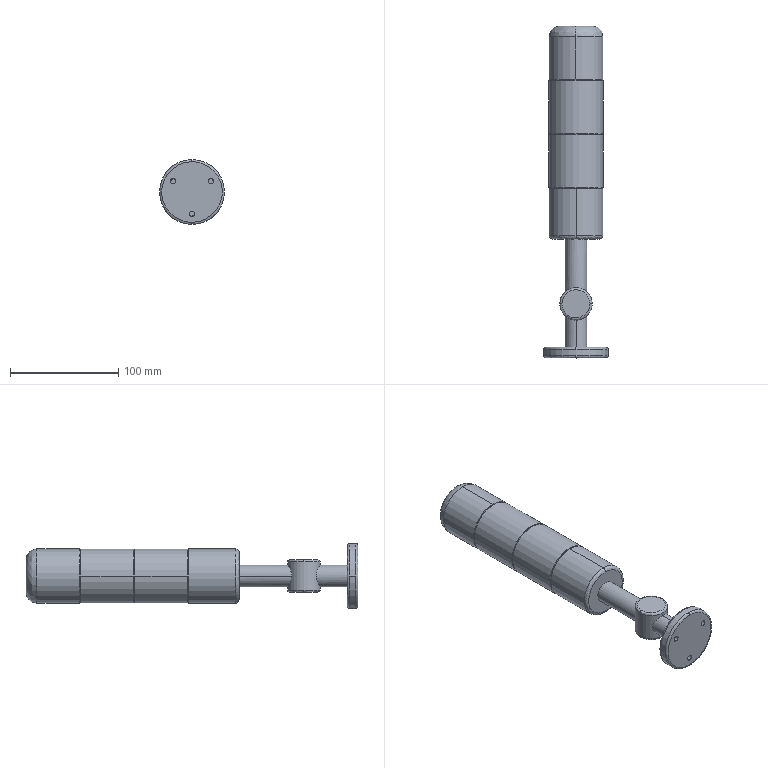Part | SolidWorks | features BaseBody 1 | 1 solid | 52 faces | box 60 x 307 x 60 mm | volume 453785 mm3 | cylinder 28 | spline 12 | plane 12 | commonest cylinder face diameters 50 x8 5 x6 48 x6 20 x4 30 x2 60 x2